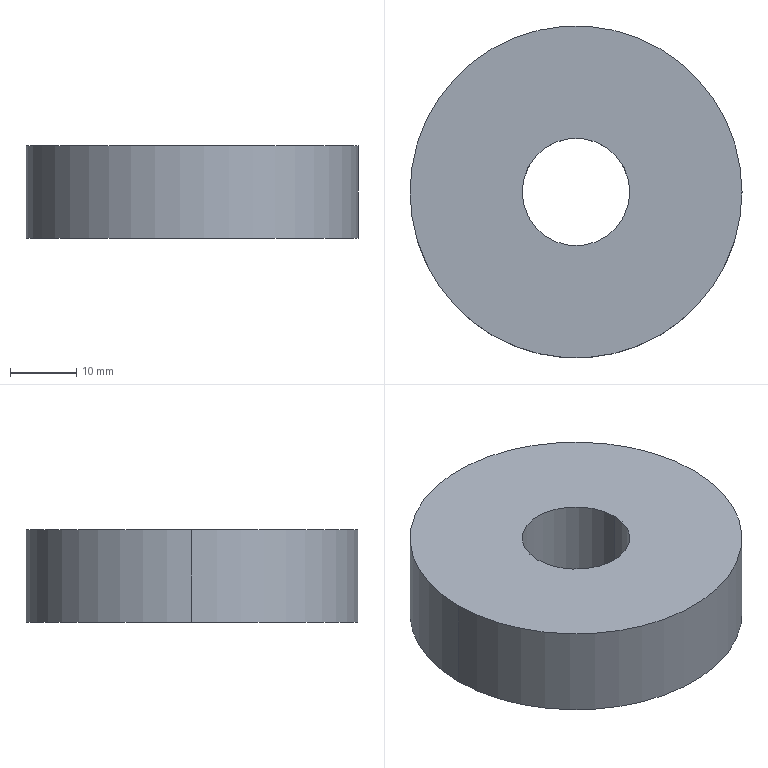Part | SolidWorks | features Extrusion 1 | 1 solid | 6 faces | box 50 x 50 x 14 mm | volume 24603 mm3 | cylinder 4 | plane 2 | commonest cylinder face diameters 16.2 x2 50 x2
STEP:
#1=CARTESIAN_POINT('',(-8.1,0.,-7.));
#2=VERTEX_POINT('',#1);
#3=CARTESIAN_POINT('',(8.1,0.,-7.));
#4=VERTEX_POINT('',#3);
#5=CARTESIAN_POINT('',(0.,0.,-7.));
#6=DIRECTION('',(0.,0.,1.));
#7=DIRECTION('',(1.,0.,0.));
#8=AXIS2_PLACEMENT_3D('',#5,#6,#7);
#9=CIRCLE('',#8,8.1);
#10=EDGE_CURVE('',#2,#4,#9,.T.);
#11=ORIENTED_EDGE('',*,*,#10,.F.);
#12=CARTESIAN_POINT('',(-8.1,0.,7.));
#13=VERTEX_POINT('',#12);
#14=CARTESIAN_POINT('',(-8.1,0.,-7.));
#15=DIRECTION('',(0.,0.,1.));
#16=VECTOR('',#15,1000.);
#17=LINE('',#14,#16);
#18=EDGE_CURVE('',#2,#13,#17,.T.);
#19=ORIENTED_EDGE('',*,*,#18,.T.);
#20=CARTESIAN_POINT('',(8.1,0.,7.));
#21=VERTEX_POINT('',#20);
#22=CARTESIAN_POINT('',(0.,0.,7.));
#23=DIRECTION('',(0.,0.,1.));
#24=DIRECTION('',(1.,0.,0.));
#25=AXIS2_PLACEMENT_3D('',#22,#23,#24);
#26=CIRCLE('',#25,8.1);
#27=EDGE_CURVE('',#13,#21,#26,.T.);
#28=ORIENTED_EDGE('',*,*,#27,.T.);
#29=CARTESIAN_POINT('',(8.1,0.,-7.));
#30=DIRECTION('',(0.,0.,1.));
#31=VECTOR('',#30,1000.);
#32=LINE('',#29,#31);
#33=EDGE_CURVE('',#4,#21,#32,.T.);
#34=ORIENTED_EDGE('',*,*,#33,.F.);
#35=EDGE_LOOP('',(#11,#19,#28,#34));
#36=FACE_OUTER_BOUND('',#35,.T.);
#37=CARTESIAN_POINT('',(0.,0.,-7.));
#38=DIRECTION('',(0.,0.,1.));
#39=DIRECTION('',(1.,0.,0.));
#40=AXIS2_PLACEMENT_3D('',#37,#38,#39);
#41=CYLINDRICAL_SURFACE('',#40,8.1);
#42=ADVANCED_FACE('',(#36),#41,.F.);
#43=CARTESIAN_POINT('',(25.,0.,-7.));
#44=VERTEX_POINT('',#43);
#45=CARTESIAN_POINT('',(-25.,0.,-7.));
#46=VERTEX_POINT('',#45);
#47=CARTESIAN_POINT('',(0.,0.,-7.));
#48=DIRECTION('',(0.,0.,1.));
#49=DIRECTION('',(1.,0.,0.));
#50=AXIS2_PLACEMENT_3D('',#47,#48,#49);
#51=CIRCLE('',#50,25.);
#52=EDGE_CURVE('',#44,#46,#51,.T.);
#53=ORIENTED_EDGE('',*,*,#52,.T.);
#54=CARTESIAN_POINT('',(-25.,0.,7.));
#55=VERTEX_POINT('',#54);
#56=CARTESIAN_POINT('',(-25.,0.,-7.));
#57=DIRECTION('',(0.,0.,1.));
#58=VECTOR('',#57,1000.);
#59=LINE('',#56,#58);
#60=EDGE_CURVE('',#46,#55,#59,.T.);
#61=ORIENTED_EDGE('',*,*,#60,.T.);
#62=CARTESIAN_POINT('',(25.,0.,7.));
#63=VERTEX_POINT('',#62);
#64=CARTESIAN_POINT('',(0.,0.,7.));
#65=DIRECTION('',(0.,0.,1.));
#66=DIRECTION('',(1.,0.,0.));
#67=AXIS2_PLACEMENT_3D('',#64,#65,#66);
#68=CIRCLE('',#67,25.);
#69=EDGE_CURVE('',#63,#55,#68,.T.);
#70=ORIENTED_EDGE('',*,*,#69,.F.);
#71=CARTESIAN_POINT('',(25.,0.,-7.));
#72=DIRECTION('',(0.,0.,1.));
#73=VECTOR('',#72,1000.);
#74=LINE('',#71,#73);
#75=EDGE_CURVE('',#44,#63,#74,.T.);
#76=ORIENTED_EDGE('',*,*,#75,.F.);
#77=EDGE_LOOP('',(#53,#61,#70,#76));
#78=FACE_OUTER_BOUND('',#77,.T.);
#79=CARTESIAN_POINT('',(0.,0.,-7.));
#80=DIRECTION('',(0.,0.,1.));
#81=DIRECTION('',(1.,0.,0.));
#82=AXIS2_PLACEMENT_3D('',#79,#80,#81);
#83=CYLINDRICAL_SURFACE('',#82,25.);
#84=ADVANCED_FACE('',(#78),#83,.T.);
#85=ORIENTED_EDGE('',*,*,#60,.F.);
#86=CARTESIAN_POINT('',(0.,0.,-7.));
#87=DIRECTION('',(0.,0.,1.));
#88=DIRECTION('',(1.,0.,0.));
#89=AXIS2_PLACEMENT_3D('',#86,#87,#88);
#90=CIRCLE('',#89,25.);
#91=EDGE_CURVE('',#46,#44,#90,.T.);
#92=ORIENTED_EDGE('',*,*,#91,.T.);
#93=ORIENTED_EDGE('',*,*,#75,.T.);
#94=CARTESIAN_POINT('',(0.,0.,7.));
#95=DIRECTION('',(0.,0.,1.));
#96=DIRECTION('',(1.,0.,0.));
#97=AXIS2_PLACEMENT_3D('',#94,#95,#96);
#98=CIRCLE('',#97,25.);
#99=EDGE_CURVE('',#55,#63,#98,.T.);
#100=ORIENTED_EDGE('',*,*,#99,.F.);
#101=EDGE_LOOP('',(#85,#92,#93,#100));
#102=FACE_OUTER_BOUND('',#101,.T.);
#103=CARTESIAN_POINT('',(0.,0.,-7.));
#104=DIRECTION('',(0.,0.,1.));
#105=DIRECTION('',(1.,0.,0.));
#106=AXIS2_PLACEMENT_3D('',#103,#104,#105);
#107=CYLINDRICAL_SURFACE('',#106,25.);
#108=ADVANCED_FACE('',(#102),#107,.T.);
#109=CARTESIAN_POINT('',(0.,0.,-7.));
#110=DIRECTION('',(0.,0.,1.));
#111=DIRECTION('',(1.,0.,0.));
#112=AXIS2_PLACEMENT_3D('',#109,#110,#111);
#113=CIRCLE('',#112,8.1);
#114=EDGE_CURVE('',#4,#2,#113,.T.);
#115=ORIENTED_EDGE('',*,*,#114,.T.);
#116=ORIENTED_EDGE('',*,*,#10,.T.);
#117=EDGE_LOOP('',(#115,#116));
#118=FACE_BOUND('',#117,.T.);
#119=ORIENTED_EDGE('',*,*,#52,.F.);
#120=ORIENTED_EDGE('',*,*,#91,.F.);
#121=EDGE_LOOP('',(#119,#120));
#122=FACE_OUTER_BOUND('',#121,.T.);
#123=CARTESIAN_POINT('',(0.,0.,-7.));
#124=DIRECTION('',(0.,0.,1.));
#125=DIRECTION('',(1.,0.,0.));
#126=AXIS2_PLACEMENT_3D('',#123,#124,#125);
#127=PLANE('',#126);
#128=ADVANCED_FACE('',(#118,#122),#127,.F.);
#129=CARTESIAN_POINT('',(0.,0.,7.));
#130=DIRECTION('',(0.,0.,1.));
#131=DIRECTION('',(1.,0.,0.));
#132=AXIS2_PLACEMENT_3D('',#129,#130,#131);
#133=CIRCLE('',#132,8.1);
#134=EDGE_CURVE('',#21,#13,#133,.T.);
#135=ORIENTED_EDGE('',*,*,#134,.F.);
#136=ORIENTED_EDGE('',*,*,#27,.F.);
#137=EDGE_LOOP('',(#135,#136));
#138=FACE_BOUND('',#137,.T.);
#139=ORIENTED_EDGE('',*,*,#69,.T.);
#140=ORIENTED_EDGE('',*,*,#99,.T.);
#141=EDGE_LOOP('',(#139,#140));
#142=FACE_OUTER_BOUND('',#141,.T.);
#143=CARTESIAN_POINT('',(0.,0.,7.));
#144=DIRECTION('',(0.,0.,1.));
#145=DIRECTION('',(1.,0.,0.));
#146=AXIS2_PLACEMENT_3D('',#143,#144,#145);
#147=PLANE('',#146);
#148=ADVANCED_FACE('',(#138,#142),#147,.T.);
#149=ORIENTED_EDGE('',*,*,#18,.F.);
#150=ORIENTED_EDGE('',*,*,#114,.F.);
#151=ORIENTED_EDGE('',*,*,#33,.T.);
#152=ORIENTED_EDGE('',*,*,#134,.T.);
#153=EDGE_LOOP('',(#149,#150,#151,#152));
#154=FACE_OUTER_BOUND('',#153,.T.);
#155=CARTESIAN_POINT('',(0.,0.,-7.));
#156=DIRECTION('',(0.,0.,1.));
#157=DIRECTION('',(1.,0.,0.));
#158=AXIS2_PLACEMENT_3D('',#155,#156,#157);
#159=CYLINDRICAL_SURFACE('',#158,8.1);
#160=ADVANCED_FACE('',(#154),#159,.F.);
#161=CLOSED_SHELL('',(#42,#84,#108,#128,#148,#160));
#162=MANIFOLD_SOLID_BREP('',#161);
#163=CARTESIAN_POINT('',(0.,0.,0.));
#164=DIRECTION('',(0.,0.,1.));
#165=DIRECTION('',(1.,0.,0.));
#166=AXIS2_PLACEMENT_3D('',#163,#164,#165);
#167=(LENGTH_UNIT()NAMED_UNIT(*)SI_UNIT(.MILLI.,.METRE.));
#168=UNCERTAINTY_MEASURE_WITH_UNIT(LENGTH_MEASURE(0.00001),#167,'','');
#169=(NAMED_UNIT(*)PLANE_ANGLE_UNIT()SI_UNIT($,.RADIAN.));
#170=(NAMED_UNIT(*)SI_UNIT($,.STERADIAN.)SOLID_ANGLE_UNIT());
#171=(GEOMETRIC_REPRESENTATION_CONTEXT(3)GLOBAL_UNCERTAINTY_ASSIGNED_CONTEXT((#168))GLOBAL_UNIT_ASSIGNED_CONTEXT((#167,#169,#170))REPRESENTATION_CONTEXT('',''));
#172=ADVANCED_BREP_SHAPE_REPRESENTATION('',(#162,#166),#171);